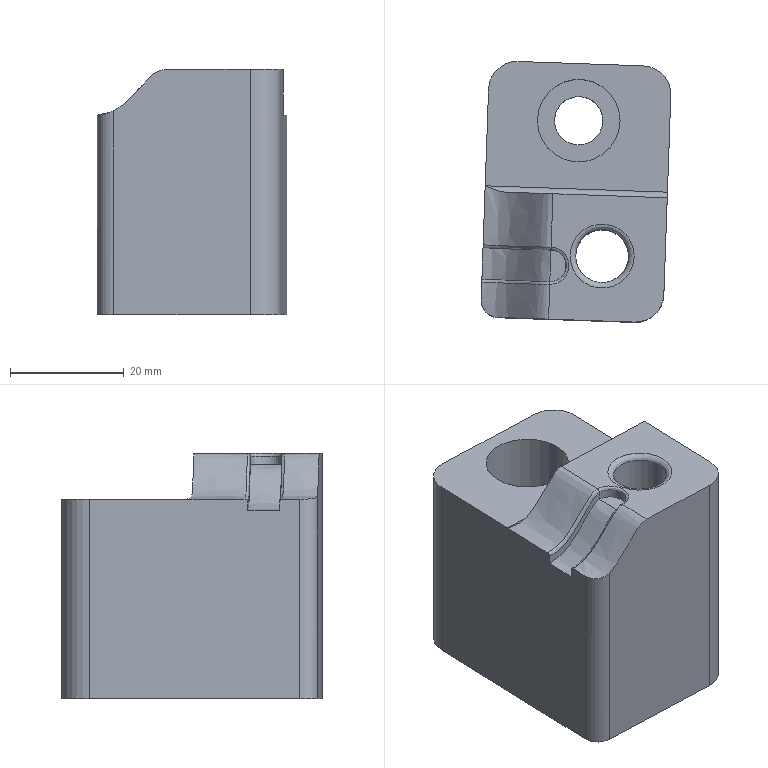Part | NX | features DIE-60 2 | 1 solid | 31 faces | box 33.277 x 45.746 x 43 mm | volume 47037 mm3 | plane 11 | spline 10 | cylinder 9 | torus 1 | commonest cylinder face diameters 10 x3 2 x1 6 x1 8.5 x1 9.27 x1 14 x1